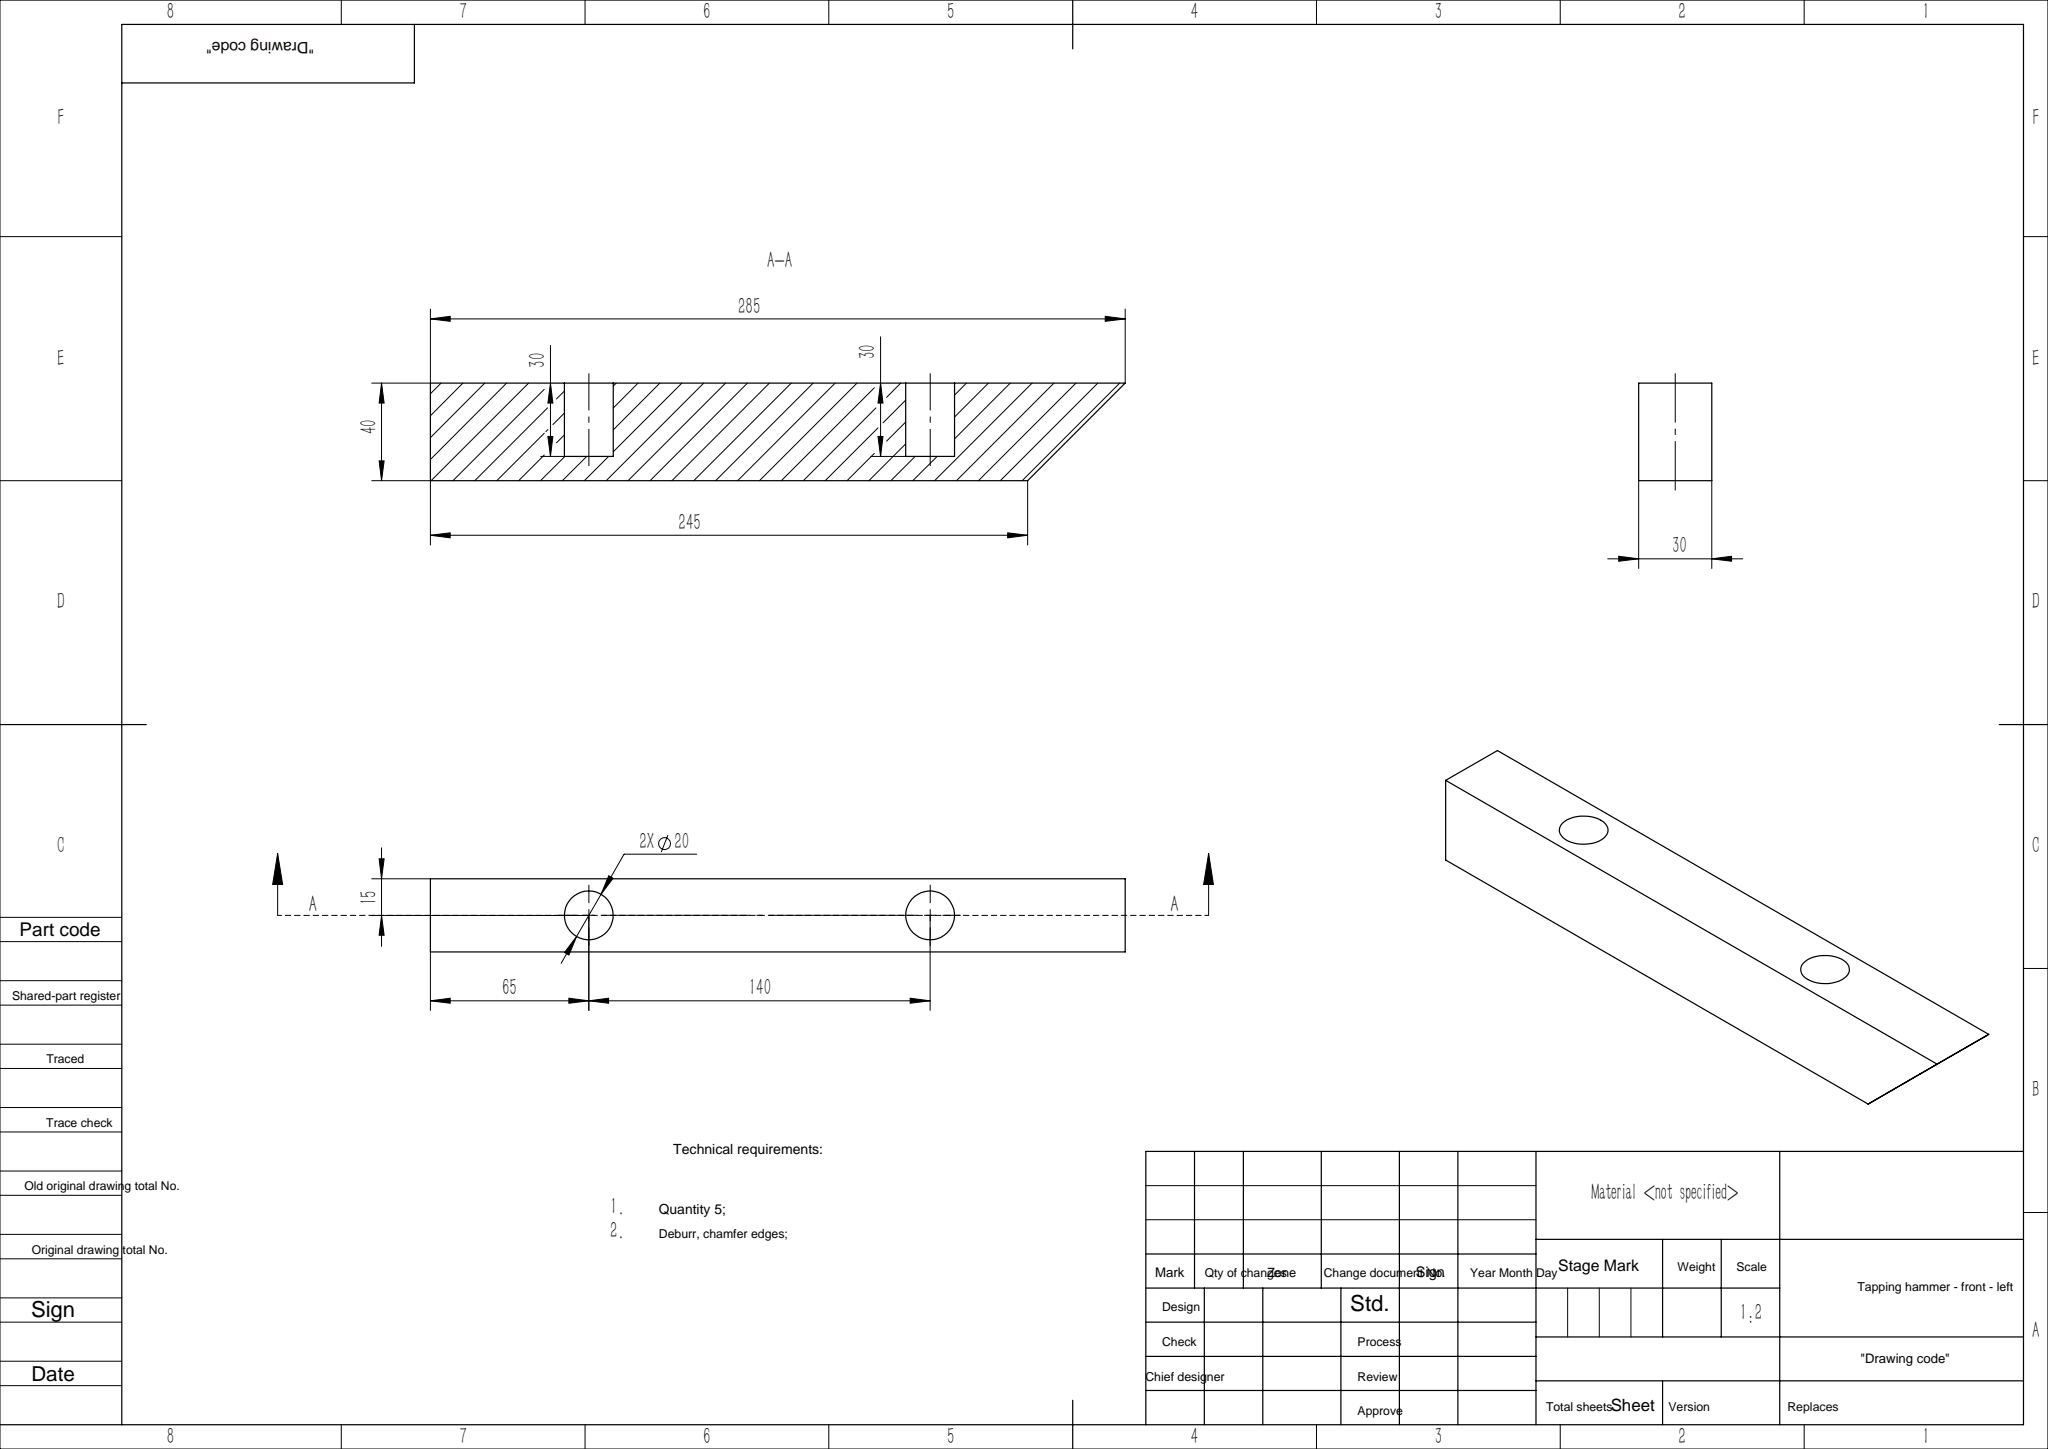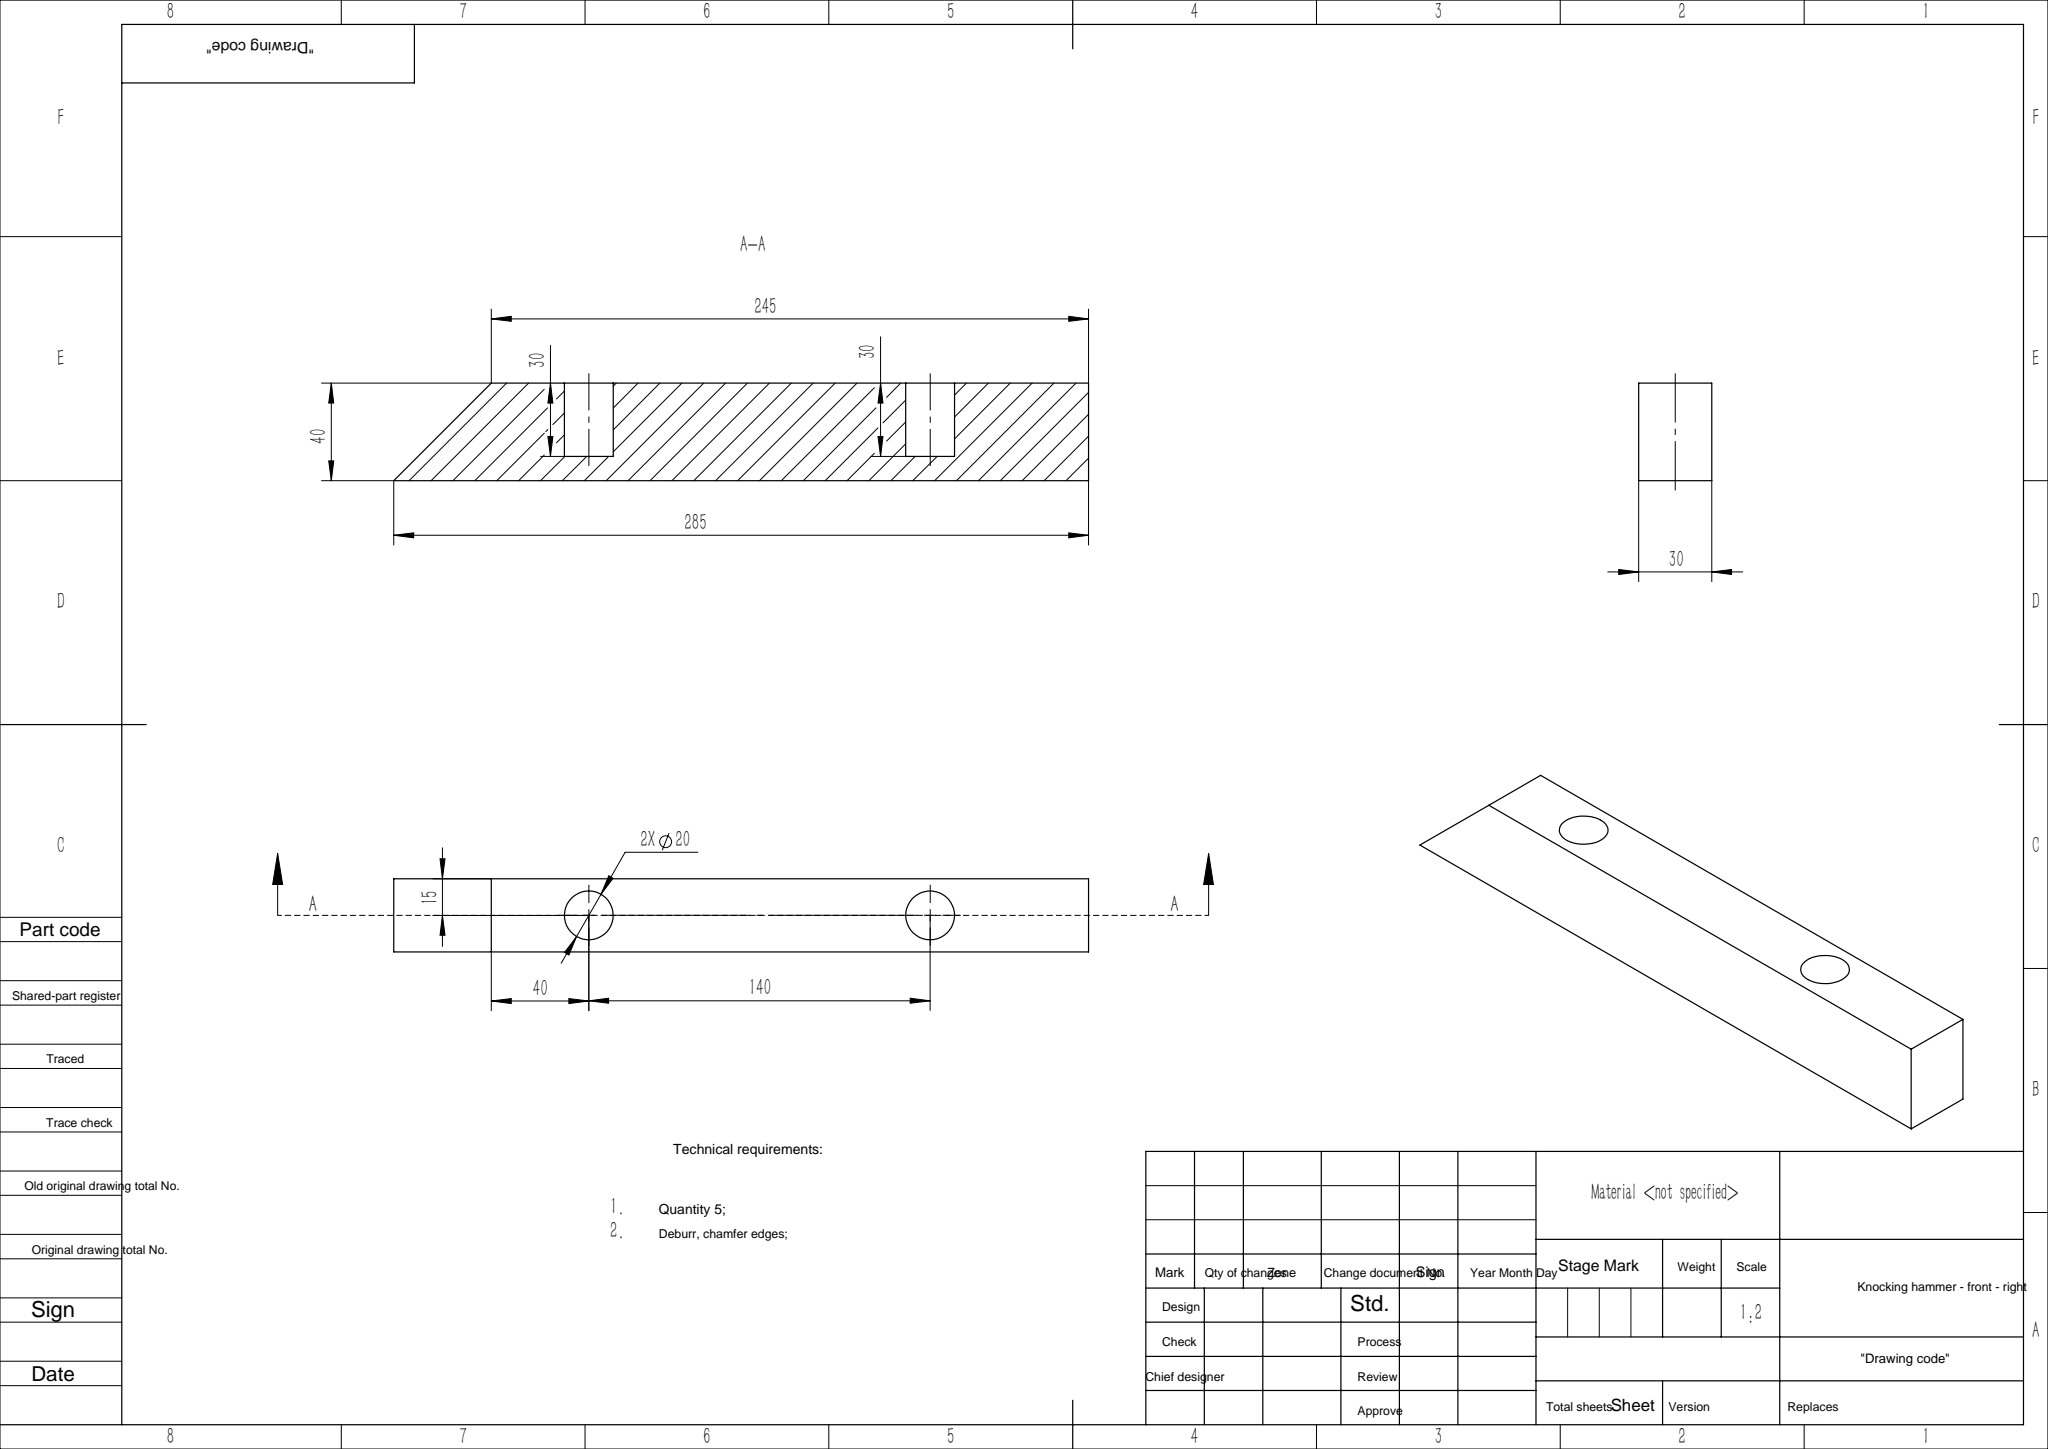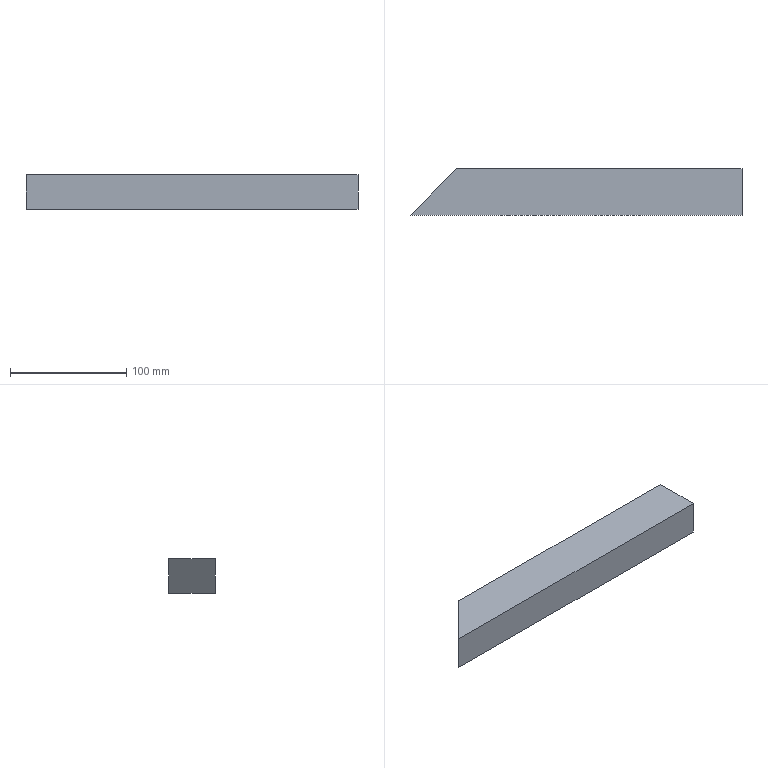Part | SolidWorks | features ICE 3, Extrusion 1 | 1 solid | 12 faces | box 285 x 40 x 30 mm | volume 299150 mm3 | plane 8 | cylinder 4 | commonest cylinder face diameters 20 x4
STEP:
#1=CARTESIAN_POINT('',(-70.,10.,-10.));
#2=VERTEX_POINT('',#1);
#3=CARTESIAN_POINT('',(-70.,10.,10.));
#4=VERTEX_POINT('',#3);
#5=CARTESIAN_POINT('',(-70.,10.,0.));
#6=DIRECTION('',(0.,1.,0.));
#7=DIRECTION('',(0.,0.,-1.));
#8=AXIS2_PLACEMENT_3D('',#5,#6,#7);
#9=CIRCLE('',#8,10.);
#10=EDGE_CURVE('',#2,#4,#9,.T.);
#11=ORIENTED_EDGE('',*,*,#10,.F.);
#12=CARTESIAN_POINT('',(-70.,40.,-10.));
#13=VERTEX_POINT('',#12);
#14=CARTESIAN_POINT('',(-70.,10.,-10.));
#15=DIRECTION('',(0.,1.,0.));
#16=VECTOR('',#15,1000.);
#17=LINE('',#14,#16);
#18=EDGE_CURVE('',#2,#13,#17,.T.);
#19=ORIENTED_EDGE('',*,*,#18,.T.);
#20=CARTESIAN_POINT('',(-70.,40.,10.));
#21=VERTEX_POINT('',#20);
#22=CARTESIAN_POINT('',(-70.,40.,0.));
#23=DIRECTION('',(0.,1.,0.));
#24=DIRECTION('',(0.,0.,-1.));
#25=AXIS2_PLACEMENT_3D('',#22,#23,#24);
#26=CIRCLE('',#25,10.);
#27=EDGE_CURVE('',#13,#21,#26,.T.);
#28=ORIENTED_EDGE('',*,*,#27,.T.);
#29=CARTESIAN_POINT('',(-70.,10.,10.));
#30=DIRECTION('',(0.,1.,0.));
#31=VECTOR('',#30,1000.);
#32=LINE('',#29,#31);
#33=EDGE_CURVE('',#4,#21,#32,.T.);
#34=ORIENTED_EDGE('',*,*,#33,.F.);
#35=EDGE_LOOP('',(#11,#19,#28,#34));
#36=FACE_OUTER_BOUND('',#35,.T.);
#37=CARTESIAN_POINT('',(-70.,10.,0.));
#38=DIRECTION('',(0.,1.,0.));
#39=DIRECTION('',(0.,0.,1.));
#40=AXIS2_PLACEMENT_3D('',#37,#38,#39);
#41=CYLINDRICAL_SURFACE('',#40,10.);
#42=ADVANCED_FACE('',(#36),#41,.F.);
#43=CARTESIAN_POINT('',(70.,10.,-10.));
#44=VERTEX_POINT('',#43);
#45=CARTESIAN_POINT('',(70.,10.,10.));
#46=VERTEX_POINT('',#45);
#47=CARTESIAN_POINT('',(70.,10.,0.));
#48=DIRECTION('',(0.,1.,0.));
#49=DIRECTION('',(0.,0.,1.));
#50=AXIS2_PLACEMENT_3D('',#47,#48,#49);
#51=CIRCLE('',#50,10.);
#52=EDGE_CURVE('',#44,#46,#51,.T.);
#53=ORIENTED_EDGE('',*,*,#52,.F.);
#54=CARTESIAN_POINT('',(70.,40.,-10.));
#55=VERTEX_POINT('',#54);
#56=CARTESIAN_POINT('',(70.,10.,-10.));
#57=DIRECTION('',(0.,1.,0.));
#58=VECTOR('',#57,1000.);
#59=LINE('',#56,#58);
#60=EDGE_CURVE('',#44,#55,#59,.T.);
#61=ORIENTED_EDGE('',*,*,#60,.T.);
#62=CARTESIAN_POINT('',(70.,40.,10.));
#63=VERTEX_POINT('',#62);
#64=CARTESIAN_POINT('',(70.,40.,0.));
#65=DIRECTION('',(0.,1.,0.));
#66=DIRECTION('',(0.,0.,1.));
#67=AXIS2_PLACEMENT_3D('',#64,#65,#66);
#68=CIRCLE('',#67,10.);
#69=EDGE_CURVE('',#55,#63,#68,.T.);
#70=ORIENTED_EDGE('',*,*,#69,.T.);
#71=CARTESIAN_POINT('',(70.,10.,10.));
#72=DIRECTION('',(0.,1.,0.));
#73=VECTOR('',#72,1000.);
#74=LINE('',#71,#73);
#75=EDGE_CURVE('',#46,#63,#74,.T.);
#76=ORIENTED_EDGE('',*,*,#75,.F.);
#77=EDGE_LOOP('',(#53,#61,#70,#76));
#78=FACE_OUTER_BOUND('',#77,.T.);
#79=CARTESIAN_POINT('',(70.,10.,0.));
#80=DIRECTION('',(0.,1.,0.));
#81=DIRECTION('',(0.,0.,1.));
#82=AXIS2_PLACEMENT_3D('',#79,#80,#81);
#83=CYLINDRICAL_SURFACE('',#82,10.);
#84=ADVANCED_FACE('',(#78),#83,.F.);
#85=CARTESIAN_POINT('',(135.,0.,15.));
#86=VERTEX_POINT('',#85);
#87=CARTESIAN_POINT('',(135.,0.,-15.));
#88=VERTEX_POINT('',#87);
#89=CARTESIAN_POINT('',(135.,0.,15.));
#90=DIRECTION('',(0.,0.,-1.));
#91=VECTOR('',#90,1000.);
#92=LINE('',#89,#91);
#93=EDGE_CURVE('',#86,#88,#92,.T.);
#94=ORIENTED_EDGE('',*,*,#93,.T.);
#95=CARTESIAN_POINT('',(135.,40.,-15.));
#96=VERTEX_POINT('',#95);
#97=CARTESIAN_POINT('',(135.,40.,-15.));
#98=DIRECTION('',(0.,-1.,0.));
#99=VECTOR('',#98,1000.);
#100=LINE('',#97,#99);
#101=EDGE_CURVE('',#96,#88,#100,.T.);
#102=ORIENTED_EDGE('',*,*,#101,.F.);
#103=CARTESIAN_POINT('',(135.,40.,15.));
#104=VERTEX_POINT('',#103);
#105=CARTESIAN_POINT('',(135.,40.,15.));
#106=DIRECTION('',(0.,0.,-1.));
#107=VECTOR('',#106,1000.);
#108=LINE('',#105,#107);
#109=EDGE_CURVE('',#104,#96,#108,.T.);
#110=ORIENTED_EDGE('',*,*,#109,.F.);
#111=CARTESIAN_POINT('',(135.,40.,15.));
#112=DIRECTION('',(0.,-1.,0.));
#113=VECTOR('',#112,1000.);
#114=LINE('',#111,#113);
#115=EDGE_CURVE('',#104,#86,#114,.T.);
#116=ORIENTED_EDGE('',*,*,#115,.T.);
#117=EDGE_LOOP('',(#94,#102,#110,#116));
#118=FACE_OUTER_BOUND('',#117,.T.);
#119=CARTESIAN_POINT('',(135.,40.,15.));
#120=DIRECTION('',(-1.,0.,0.));
#121=DIRECTION('',(0.,0.,1.));
#122=AXIS2_PLACEMENT_3D('',#119,#120,#121);
#123=PLANE('',#122);
#124=ADVANCED_FACE('',(#118),#123,.F.);
#125=CARTESIAN_POINT('',(-150.,0.,-15.));
#126=VERTEX_POINT('',#125);
#127=CARTESIAN_POINT('',(-135.,0.,-15.));
#128=DIRECTION('',(-1.,0.,0.));
#129=VECTOR('',#128,1000.);
#130=LINE('',#127,#129);
#131=EDGE_CURVE('',#88,#126,#130,.T.);
#132=ORIENTED_EDGE('',*,*,#131,.T.);
#133=CARTESIAN_POINT('',(-110.,40.,-15.));
#134=VERTEX_POINT('',#133);
#135=CARTESIAN_POINT('',(-150.,0.,-15.));
#136=DIRECTION('',(0.7071,0.7071,0.));
#137=VECTOR('',#136,1000.);
#138=LINE('',#135,#137);
#139=EDGE_CURVE('',#126,#134,#138,.T.);
#140=ORIENTED_EDGE('',*,*,#139,.T.);
#141=CARTESIAN_POINT('',(-135.,40.,-15.));
#142=DIRECTION('',(-1.,0.,0.));
#143=VECTOR('',#142,1000.);
#144=LINE('',#141,#143);
#145=EDGE_CURVE('',#96,#134,#144,.T.);
#146=ORIENTED_EDGE('',*,*,#145,.F.);
#147=ORIENTED_EDGE('',*,*,#101,.T.);
#148=EDGE_LOOP('',(#132,#140,#146,#147));
#149=FACE_OUTER_BOUND('',#148,.T.);
#150=CARTESIAN_POINT('',(-135.,40.,-15.));
#151=DIRECTION('',(0.,0.,1.));
#152=DIRECTION('',(1.,0.,0.));
#153=AXIS2_PLACEMENT_3D('',#150,#151,#152);
#154=PLANE('',#153);
#155=ADVANCED_FACE('',(#149),#154,.F.);
#156=CARTESIAN_POINT('',(-110.,40.,15.));
#157=VERTEX_POINT('',#156);
#158=CARTESIAN_POINT('',(-135.,40.,15.));
#159=DIRECTION('',(1.,0.,0.));
#160=VECTOR('',#159,1000.);
#161=LINE('',#158,#160);
#162=EDGE_CURVE('',#157,#104,#161,.T.);
#163=ORIENTED_EDGE('',*,*,#162,.F.);
#164=CARTESIAN_POINT('',(-150.,0.,15.));
#165=VERTEX_POINT('',#164);
#166=CARTESIAN_POINT('',(-150.,0.,15.));
#167=DIRECTION('',(0.7071,0.7071,0.));
#168=VECTOR('',#167,1000.);
#169=LINE('',#166,#168);
#170=EDGE_CURVE('',#165,#157,#169,.T.);
#171=ORIENTED_EDGE('',*,*,#170,.F.);
#172=CARTESIAN_POINT('',(-135.,0.,15.));
#173=DIRECTION('',(1.,0.,0.));
#174=VECTOR('',#173,1000.);
#175=LINE('',#172,#174);
#176=EDGE_CURVE('',#165,#86,#175,.T.);
#177=ORIENTED_EDGE('',*,*,#176,.T.);
#178=ORIENTED_EDGE('',*,*,#115,.F.);
#179=EDGE_LOOP('',(#163,#171,#177,#178));
#180=FACE_OUTER_BOUND('',#179,.T.);
#181=CARTESIAN_POINT('',(-135.,40.,15.));
#182=DIRECTION('',(0.,0.,-1.));
#183=DIRECTION('',(-1.,0.,0.));
#184=AXIS2_PLACEMENT_3D('',#181,#182,#183);
#185=PLANE('',#184);
#186=ADVANCED_FACE('',(#180),#185,.F.);
#187=CARTESIAN_POINT('',(-70.,40.,0.));
#188=DIRECTION('',(0.,1.,0.));
#189=DIRECTION('',(0.,0.,-1.));
#190=AXIS2_PLACEMENT_3D('',#187,#188,#189);
#191=CIRCLE('',#190,10.);
#192=EDGE_CURVE('',#21,#13,#191,.T.);
#193=ORIENTED_EDGE('',*,*,#192,.F.);
#194=ORIENTED_EDGE('',*,*,#27,.F.);
#195=EDGE_LOOP('',(#193,#194));
#196=FACE_BOUND('',#195,.T.);
#197=CARTESIAN_POINT('',(70.,40.,0.));
#198=DIRECTION('',(0.,1.,0.));
#199=DIRECTION('',(0.,0.,1.));
#200=AXIS2_PLACEMENT_3D('',#197,#198,#199);
#201=CIRCLE('',#200,10.);
#202=EDGE_CURVE('',#63,#55,#201,.T.);
#203=ORIENTED_EDGE('',*,*,#202,.F.);
#204=ORIENTED_EDGE('',*,*,#69,.F.);
#205=EDGE_LOOP('',(#203,#204));
#206=FACE_BOUND('',#205,.T.);
#207=ORIENTED_EDGE('',*,*,#145,.T.);
#208=CARTESIAN_POINT('',(-110.,40.,-15.));
#209=DIRECTION('',(0.,0.,1.));
#210=VECTOR('',#209,1000.);
#211=LINE('',#208,#210);
#212=EDGE_CURVE('',#134,#157,#211,.T.);
#213=ORIENTED_EDGE('',*,*,#212,.T.);
#214=ORIENTED_EDGE('',*,*,#162,.T.);
#215=ORIENTED_EDGE('',*,*,#109,.T.);
#216=EDGE_LOOP('',(#207,#213,#214,#215));
#217=FACE_OUTER_BOUND('',#216,.T.);
#218=CARTESIAN_POINT('',(0.,40.,0.));
#219=DIRECTION('',(0.,-1.,0.));
#220=DIRECTION('',(0.,0.,-1.));
#221=AXIS2_PLACEMENT_3D('',#218,#219,#220);
#222=PLANE('',#221);
#223=ADVANCED_FACE('',(#196,#206,#217),#222,.F.);
#224=ORIENTED_EDGE('',*,*,#93,.F.);
#225=ORIENTED_EDGE('',*,*,#176,.F.);
#226=CARTESIAN_POINT('',(-150.,0.,-15.));
#227=DIRECTION('',(0.,0.,1.));
#228=VECTOR('',#227,1000.);
#229=LINE('',#226,#228);
#230=EDGE_CURVE('',#126,#165,#229,.T.);
#231=ORIENTED_EDGE('',*,*,#230,.F.);
#232=ORIENTED_EDGE('',*,*,#131,.F.);
#233=EDGE_LOOP('',(#224,#225,#231,#232));
#234=FACE_OUTER_BOUND('',#233,.T.);
#235=CARTESIAN_POINT('',(0.,0.,0.));
#236=DIRECTION('',(0.,-1.,0.));
#237=DIRECTION('',(0.,0.,-1.));
#238=AXIS2_PLACEMENT_3D('',#235,#236,#237);
#239=PLANE('',#238);
#240=ADVANCED_FACE('',(#234),#239,.T.);
#241=ORIENTED_EDGE('',*,*,#60,.F.);
#242=CARTESIAN_POINT('',(70.,10.,0.));
#243=DIRECTION('',(0.,1.,0.));
#244=DIRECTION('',(0.,0.,1.));
#245=AXIS2_PLACEMENT_3D('',#242,#243,#244);
#246=CIRCLE('',#245,10.);
#247=EDGE_CURVE('',#46,#44,#246,.T.);
#248=ORIENTED_EDGE('',*,*,#247,.F.);
#249=ORIENTED_EDGE('',*,*,#75,.T.);
#250=ORIENTED_EDGE('',*,*,#202,.T.);
#251=EDGE_LOOP('',(#241,#248,#249,#250));
#252=FACE_OUTER_BOUND('',#251,.T.);
#253=CARTESIAN_POINT('',(70.,10.,0.));
#254=DIRECTION('',(0.,1.,0.));
#255=DIRECTION('',(0.,0.,1.));
#256=AXIS2_PLACEMENT_3D('',#253,#254,#255);
#257=CYLINDRICAL_SURFACE('',#256,10.);
#258=ADVANCED_FACE('',(#252),#257,.F.);
#259=ORIENTED_EDGE('',*,*,#247,.T.);
#260=ORIENTED_EDGE('',*,*,#52,.T.);
#261=EDGE_LOOP('',(#259,#260));
#262=FACE_OUTER_BOUND('',#261,.T.);
#263=CARTESIAN_POINT('',(70.,10.,0.));
#264=DIRECTION('',(0.,1.,0.));
#265=DIRECTION('',(0.,0.,1.));
#266=AXIS2_PLACEMENT_3D('',#263,#264,#265);
#267=PLANE('',#266);
#268=ADVANCED_FACE('',(#262),#267,.T.);
#269=ORIENTED_EDGE('',*,*,#18,.F.);
#270=CARTESIAN_POINT('',(-70.,10.,0.));
#271=DIRECTION('',(0.,1.,0.));
#272=DIRECTION('',(0.,0.,-1.));
#273=AXIS2_PLACEMENT_3D('',#270,#271,#272);
#274=CIRCLE('',#273,10.);
#275=EDGE_CURVE('',#4,#2,#274,.T.);
#276=ORIENTED_EDGE('',*,*,#275,.F.);
#277=ORIENTED_EDGE('',*,*,#33,.T.);
#278=ORIENTED_EDGE('',*,*,#192,.T.);
#279=EDGE_LOOP('',(#269,#276,#277,#278));
#280=FACE_OUTER_BOUND('',#279,.T.);
#281=CARTESIAN_POINT('',(-70.,10.,0.));
#282=DIRECTION('',(0.,1.,0.));
#283=DIRECTION('',(0.,0.,1.));
#284=AXIS2_PLACEMENT_3D('',#281,#282,#283);
#285=CYLINDRICAL_SURFACE('',#284,10.);
#286=ADVANCED_FACE('',(#280),#285,.F.);
#287=ORIENTED_EDGE('',*,*,#275,.T.);
#288=ORIENTED_EDGE('',*,*,#10,.T.);
#289=EDGE_LOOP('',(#287,#288));
#290=FACE_OUTER_BOUND('',#289,.T.);
#291=CARTESIAN_POINT('',(-70.,10.,0.));
#292=DIRECTION('',(0.,-1.,0.));
#293=DIRECTION('',(0.,0.,-1.));
#294=AXIS2_PLACEMENT_3D('',#291,#292,#293);
#295=PLANE('',#294);
#296=ADVANCED_FACE('',(#290),#295,.F.);
#297=ORIENTED_EDGE('',*,*,#170,.T.);
#298=ORIENTED_EDGE('',*,*,#212,.F.);
#299=ORIENTED_EDGE('',*,*,#139,.F.);
#300=ORIENTED_EDGE('',*,*,#230,.T.);
#301=EDGE_LOOP('',(#297,#298,#299,#300));
#302=FACE_OUTER_BOUND('',#301,.T.);
#303=CARTESIAN_POINT('',(-150.,0.,-15.));
#304=DIRECTION('',(0.7071,-0.7071,0.));
#305=DIRECTION('',(0.7071,0.7071,0.));
#306=AXIS2_PLACEMENT_3D('',#303,#304,#305);
#307=PLANE('',#306);
#308=ADVANCED_FACE('',(#302),#307,.F.);
#309=CLOSED_SHELL('',(#42,#84,#124,#155,#186,#223,#240,#258,#268,#286,#296,#308));
#310=MANIFOLD_SOLID_BREP('',#309);
#311=CARTESIAN_POINT('',(0.,0.,0.));
#312=DIRECTION('',(0.,0.,1.));
#313=DIRECTION('',(1.,0.,0.));
#314=AXIS2_PLACEMENT_3D('',#311,#312,#313);
#315=(LENGTH_UNIT()NAMED_UNIT(*)SI_UNIT(.MILLI.,.METRE.));
#316=UNCERTAINTY_MEASURE_WITH_UNIT(LENGTH_MEASURE(0.00001),#315,'','');
#317=(NAMED_UNIT(*)PLANE_ANGLE_UNIT()SI_UNIT($,.RADIAN.));
#318=(NAMED_UNIT(*)SI_UNIT($,.STERADIAN.)SOLID_ANGLE_UNIT());
#319=(GEOMETRIC_REPRESENTATION_CONTEXT(3)GLOBAL_UNCERTAINTY_ASSIGNED_CONTEXT((#316))GLOBAL_UNIT_ASSIGNED_CONTEXT((#315,#317,#318))REPRESENTATION_CONTEXT('',''));
#320=ADVANCED_BREP_SHAPE_REPRESENTATION('',(#310,#314),#319);